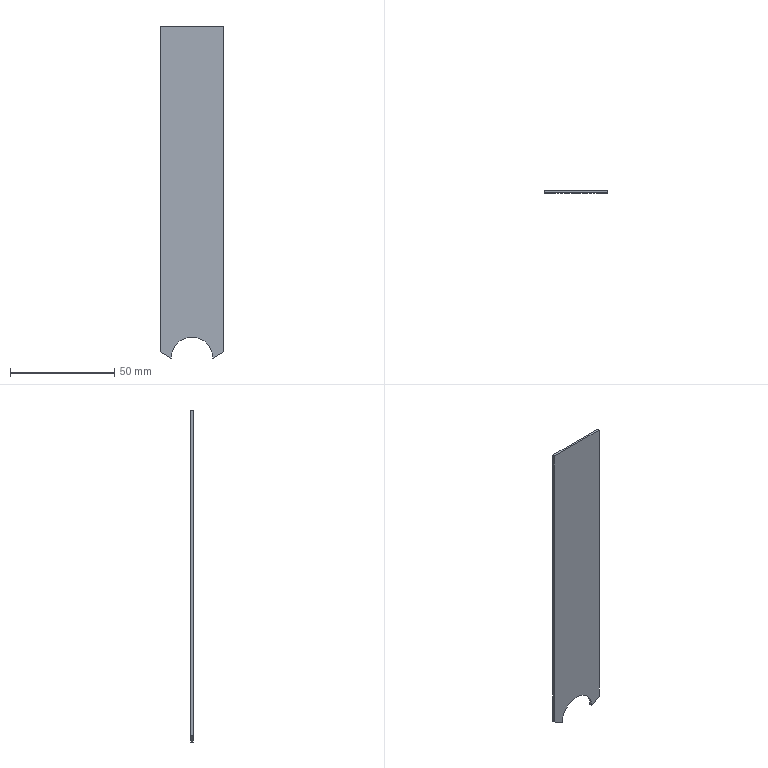Part | STEP file | solid 163 | 1 solid | 10 faces | box 30.5 x 1 x 159.425 mm | volume 4694 mm3 | plane 5 | cylinder 3 | cone 2 | commonest cylinder face diameters 30.5 x2 20 x1